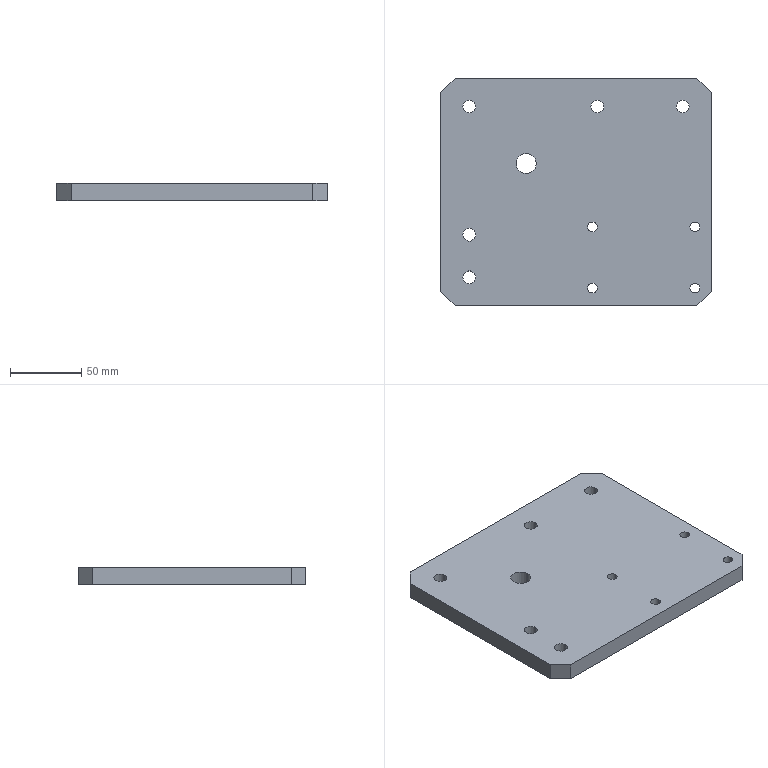Part | SolidWorks | features BaseBody 1 | 1 solid | 30 faces | box 190 x 160 x 12 mm | volume 354993 mm3 | cylinder 20 | plane 10 | commonest cylinder face diameters 9 x10 6.8 x8 14 x2
STEP:
#1=CARTESIAN_POINT('',(181.9,-147.5,15.));
#2=VERTEX_POINT('',#1);
#3=CARTESIAN_POINT('',(175.1,-147.5,15.));
#4=VERTEX_POINT('',#3);
#5=CARTESIAN_POINT('',(178.5,-147.5,15.));
#6=DIRECTION('',(0.,0.,-1.));
#7=DIRECTION('',(-1.,0.,0.));
#8=AXIS2_PLACEMENT_3D('',#5,#6,#7);
#9=CIRCLE('',#8,3.4);
#10=EDGE_CURVE('',#2,#4,#9,.T.);
#11=ORIENTED_EDGE('',*,*,#10,.F.);
#12=CARTESIAN_POINT('',(181.9,-147.5,3.));
#13=VERTEX_POINT('',#12);
#14=CARTESIAN_POINT('',(181.9,-147.5,3.));
#15=DIRECTION('',(0.,0.,-1.));
#16=VECTOR('',#15,1000.);
#17=LINE('',#14,#16);
#18=EDGE_CURVE('',#2,#13,#17,.T.);
#19=ORIENTED_EDGE('',*,*,#18,.T.);
#20=CARTESIAN_POINT('',(175.1,-147.5,3.));
#21=VERTEX_POINT('',#20);
#22=CARTESIAN_POINT('',(178.5,-147.5,3.));
#23=DIRECTION('',(0.,0.,-1.));
#24=DIRECTION('',(-1.,0.,0.));
#25=AXIS2_PLACEMENT_3D('',#22,#23,#24);
#26=CIRCLE('',#25,3.4);
#27=EDGE_CURVE('',#13,#21,#26,.T.);
#28=ORIENTED_EDGE('',*,*,#27,.T.);
#29=CARTESIAN_POINT('',(175.1,-147.5,3.));
#30=DIRECTION('',(0.,0.,-1.));
#31=VECTOR('',#30,1000.);
#32=LINE('',#29,#31);
#33=EDGE_CURVE('',#4,#21,#32,.T.);
#34=ORIENTED_EDGE('',*,*,#33,.F.);
#35=EDGE_LOOP('',(#11,#19,#28,#34));
#36=FACE_OUTER_BOUND('',#35,.T.);
#37=CARTESIAN_POINT('',(178.5,-147.5,3.));
#38=DIRECTION('',(0.,0.,-1.));
#39=DIRECTION('',(-1.,0.,0.));
#40=AXIS2_PLACEMENT_3D('',#37,#38,#39);
#41=CYLINDRICAL_SURFACE('',#40,3.4);
#42=ADVANCED_FACE('',(#36),#41,.F.);
#43=CARTESIAN_POINT('',(181.9,-104.5,15.));
#44=VERTEX_POINT('',#43);
#45=CARTESIAN_POINT('',(175.1,-104.5,15.));
#46=VERTEX_POINT('',#45);
#47=CARTESIAN_POINT('',(178.5,-104.5,15.));
#48=DIRECTION('',(0.,0.,-1.));
#49=DIRECTION('',(-1.,0.,0.));
#50=AXIS2_PLACEMENT_3D('',#47,#48,#49);
#51=CIRCLE('',#50,3.4);
#52=EDGE_CURVE('',#44,#46,#51,.T.);
#53=ORIENTED_EDGE('',*,*,#52,.F.);
#54=CARTESIAN_POINT('',(181.9,-104.5,3.));
#55=VERTEX_POINT('',#54);
#56=CARTESIAN_POINT('',(181.9,-104.5,3.));
#57=DIRECTION('',(0.,0.,-1.));
#58=VECTOR('',#57,1000.);
#59=LINE('',#56,#58);
#60=EDGE_CURVE('',#44,#55,#59,.T.);
#61=ORIENTED_EDGE('',*,*,#60,.T.);
#62=CARTESIAN_POINT('',(175.1,-104.5,3.));
#63=VERTEX_POINT('',#62);
#64=CARTESIAN_POINT('',(178.5,-104.5,3.));
#65=DIRECTION('',(0.,0.,-1.));
#66=DIRECTION('',(-1.,0.,0.));
#67=AXIS2_PLACEMENT_3D('',#64,#65,#66);
#68=CIRCLE('',#67,3.4);
#69=EDGE_CURVE('',#55,#63,#68,.T.);
#70=ORIENTED_EDGE('',*,*,#69,.T.);
#71=CARTESIAN_POINT('',(175.1,-104.5,3.));
#72=DIRECTION('',(0.,0.,-1.));
#73=VECTOR('',#72,1000.);
#74=LINE('',#71,#73);
#75=EDGE_CURVE('',#46,#63,#74,.T.);
#76=ORIENTED_EDGE('',*,*,#75,.F.);
#77=EDGE_LOOP('',(#53,#61,#70,#76));
#78=FACE_OUTER_BOUND('',#77,.T.);
#79=CARTESIAN_POINT('',(178.5,-104.5,3.));
#80=DIRECTION('',(0.,0.,-1.));
#81=DIRECTION('',(-1.,0.,0.));
#82=AXIS2_PLACEMENT_3D('',#79,#80,#81);
#83=CYLINDRICAL_SURFACE('',#82,3.4);
#84=ADVANCED_FACE('',(#78),#83,.F.);
#85=CARTESIAN_POINT('',(109.9,-104.5,15.));
#86=VERTEX_POINT('',#85);
#87=CARTESIAN_POINT('',(103.1,-104.5,15.));
#88=VERTEX_POINT('',#87);
#89=CARTESIAN_POINT('',(106.5,-104.5,15.));
#90=DIRECTION('',(0.,0.,-1.));
#91=DIRECTION('',(-1.,0.,0.));
#92=AXIS2_PLACEMENT_3D('',#89,#90,#91);
#93=CIRCLE('',#92,3.4);
#94=EDGE_CURVE('',#86,#88,#93,.T.);
#95=ORIENTED_EDGE('',*,*,#94,.F.);
#96=CARTESIAN_POINT('',(109.9,-104.5,3.));
#97=VERTEX_POINT('',#96);
#98=CARTESIAN_POINT('',(109.9,-104.5,3.));
#99=DIRECTION('',(0.,0.,-1.));
#100=VECTOR('',#99,1000.);
#101=LINE('',#98,#100);
#102=EDGE_CURVE('',#86,#97,#101,.T.);
#103=ORIENTED_EDGE('',*,*,#102,.T.);
#104=CARTESIAN_POINT('',(103.1,-104.5,3.));
#105=VERTEX_POINT('',#104);
#106=CARTESIAN_POINT('',(106.5,-104.5,3.));
#107=DIRECTION('',(0.,0.,-1.));
#108=DIRECTION('',(-1.,0.,0.));
#109=AXIS2_PLACEMENT_3D('',#106,#107,#108);
#110=CIRCLE('',#109,3.4);
#111=EDGE_CURVE('',#97,#105,#110,.T.);
#112=ORIENTED_EDGE('',*,*,#111,.T.);
#113=CARTESIAN_POINT('',(103.1,-104.5,3.));
#114=DIRECTION('',(0.,0.,-1.));
#115=VECTOR('',#114,1000.);
#116=LINE('',#113,#115);
#117=EDGE_CURVE('',#88,#105,#116,.T.);
#118=ORIENTED_EDGE('',*,*,#117,.F.);
#119=EDGE_LOOP('',(#95,#103,#112,#118));
#120=FACE_OUTER_BOUND('',#119,.T.);
#121=CARTESIAN_POINT('',(106.5,-104.5,3.));
#122=DIRECTION('',(0.,0.,-1.));
#123=DIRECTION('',(-1.,0.,0.));
#124=AXIS2_PLACEMENT_3D('',#121,#122,#123);
#125=CYLINDRICAL_SURFACE('',#124,3.4);
#126=ADVANCED_FACE('',(#120),#125,.F.);
#127=CARTESIAN_POINT('',(109.9,-147.5,15.));
#128=VERTEX_POINT('',#127);
#129=CARTESIAN_POINT('',(103.1,-147.5,15.));
#130=VERTEX_POINT('',#129);
#131=CARTESIAN_POINT('',(106.5,-147.5,15.));
#132=DIRECTION('',(0.,0.,-1.));
#133=DIRECTION('',(-1.,0.,0.));
#134=AXIS2_PLACEMENT_3D('',#131,#132,#133);
#135=CIRCLE('',#134,3.4);
#136=EDGE_CURVE('',#128,#130,#135,.T.);
#137=ORIENTED_EDGE('',*,*,#136,.F.);
#138=CARTESIAN_POINT('',(109.9,-147.5,3.));
#139=VERTEX_POINT('',#138);
#140=CARTESIAN_POINT('',(109.9,-147.5,3.));
#141=DIRECTION('',(0.,0.,-1.));
#142=VECTOR('',#141,1000.);
#143=LINE('',#140,#142);
#144=EDGE_CURVE('',#128,#139,#143,.T.);
#145=ORIENTED_EDGE('',*,*,#144,.T.);
#146=CARTESIAN_POINT('',(103.1,-147.5,3.));
#147=VERTEX_POINT('',#146);
#148=CARTESIAN_POINT('',(106.5,-147.5,3.));
#149=DIRECTION('',(0.,0.,-1.));
#150=DIRECTION('',(-1.,0.,0.));
#151=AXIS2_PLACEMENT_3D('',#148,#149,#150);
#152=CIRCLE('',#151,3.4);
#153=EDGE_CURVE('',#139,#147,#152,.T.);
#154=ORIENTED_EDGE('',*,*,#153,.T.);
#155=CARTESIAN_POINT('',(103.1,-147.5,3.));
#156=DIRECTION('',(0.,0.,-1.));
#157=VECTOR('',#156,1000.);
#158=LINE('',#155,#157);
#159=EDGE_CURVE('',#130,#147,#158,.T.);
#160=ORIENTED_EDGE('',*,*,#159,.F.);
#161=EDGE_LOOP('',(#137,#145,#154,#160));
#162=FACE_OUTER_BOUND('',#161,.T.);
#163=CARTESIAN_POINT('',(106.5,-147.5,3.));
#164=DIRECTION('',(0.,0.,-1.));
#165=DIRECTION('',(-1.,0.,0.));
#166=AXIS2_PLACEMENT_3D('',#163,#164,#165);
#167=CYLINDRICAL_SURFACE('',#166,3.4);
#168=ADVANCED_FACE('',(#162),#167,.F.);
#169=CARTESIAN_POINT('',(67.,-60.,15.));
#170=VERTEX_POINT('',#169);
#171=CARTESIAN_POINT('',(53.,-60.,15.));
#172=VERTEX_POINT('',#171);
#173=CARTESIAN_POINT('',(60.,-60.,15.));
#174=DIRECTION('',(0.,0.,-1.));
#175=DIRECTION('',(-1.,0.,0.));
#176=AXIS2_PLACEMENT_3D('',#173,#174,#175);
#177=CIRCLE('',#176,7.);
#178=EDGE_CURVE('',#170,#172,#177,.T.);
#179=ORIENTED_EDGE('',*,*,#178,.F.);
#180=CARTESIAN_POINT('',(67.,-60.,3.));
#181=VERTEX_POINT('',#180);
#182=CARTESIAN_POINT('',(67.,-60.,3.));
#183=DIRECTION('',(0.,0.,-1.));
#184=VECTOR('',#183,1000.);
#185=LINE('',#182,#184);
#186=EDGE_CURVE('',#170,#181,#185,.T.);
#187=ORIENTED_EDGE('',*,*,#186,.T.);
#188=CARTESIAN_POINT('',(53.,-60.,3.));
#189=VERTEX_POINT('',#188);
#190=CARTESIAN_POINT('',(60.,-60.,3.));
#191=DIRECTION('',(0.,0.,-1.));
#192=DIRECTION('',(-1.,0.,0.));
#193=AXIS2_PLACEMENT_3D('',#190,#191,#192);
#194=CIRCLE('',#193,7.);
#195=EDGE_CURVE('',#181,#189,#194,.T.);
#196=ORIENTED_EDGE('',*,*,#195,.T.);
#197=CARTESIAN_POINT('',(53.,-60.,3.));
#198=DIRECTION('',(0.,0.,-1.));
#199=VECTOR('',#198,1000.);
#200=LINE('',#197,#199);
#201=EDGE_CURVE('',#172,#189,#200,.T.);
#202=ORIENTED_EDGE('',*,*,#201,.F.);
#203=EDGE_LOOP('',(#179,#187,#196,#202));
#204=FACE_OUTER_BOUND('',#203,.T.);
#205=CARTESIAN_POINT('',(60.,-60.,3.));
#206=DIRECTION('',(0.,0.,-1.));
#207=DIRECTION('',(-1.,0.,0.));
#208=AXIS2_PLACEMENT_3D('',#205,#206,#207);
#209=CYLINDRICAL_SURFACE('',#208,7.);
#210=ADVANCED_FACE('',(#204),#209,.F.);
#211=CARTESIAN_POINT('',(15.5,-20.,3.));
#212=VERTEX_POINT('',#211);
#213=CARTESIAN_POINT('',(24.5,-20.,3.));
#214=VERTEX_POINT('',#213);
#215=CARTESIAN_POINT('',(20.,-20.,3.));
#216=DIRECTION('',(0.,0.,1.));
#217=DIRECTION('',(1.,0.,0.));
#218=AXIS2_PLACEMENT_3D('',#215,#216,#217);
#219=CIRCLE('',#218,4.5);
#220=EDGE_CURVE('',#212,#214,#219,.T.);
#221=ORIENTED_EDGE('',*,*,#220,.F.);
#222=CARTESIAN_POINT('',(15.5,-20.,15.));
#223=VERTEX_POINT('',#222);
#224=CARTESIAN_POINT('',(15.5,-20.,15.));
#225=DIRECTION('',(0.,0.,1.));
#226=VECTOR('',#225,1000.);
#227=LINE('',#224,#226);
#228=EDGE_CURVE('',#212,#223,#227,.T.);
#229=ORIENTED_EDGE('',*,*,#228,.T.);
#230=CARTESIAN_POINT('',(24.5,-20.,15.));
#231=VERTEX_POINT('',#230);
#232=CARTESIAN_POINT('',(20.,-20.,15.));
#233=DIRECTION('',(0.,0.,1.));
#234=DIRECTION('',(1.,0.,0.));
#235=AXIS2_PLACEMENT_3D('',#232,#233,#234);
#236=CIRCLE('',#235,4.5);
#237=EDGE_CURVE('',#223,#231,#236,.T.);
#238=ORIENTED_EDGE('',*,*,#237,.T.);
#239=CARTESIAN_POINT('',(24.5,-20.,15.));
#240=DIRECTION('',(0.,0.,1.));
#241=VECTOR('',#240,1000.);
#242=LINE('',#239,#241);
#243=EDGE_CURVE('',#214,#231,#242,.T.);
#244=ORIENTED_EDGE('',*,*,#243,.F.);
#245=EDGE_LOOP('',(#221,#229,#238,#244));
#246=FACE_OUTER_BOUND('',#245,.T.);
#247=CARTESIAN_POINT('',(20.,-20.,15.));
#248=DIRECTION('',(0.,0.,1.));
#249=DIRECTION('',(1.,0.,0.));
#250=AXIS2_PLACEMENT_3D('',#247,#248,#249);
#251=CYLINDRICAL_SURFACE('',#250,4.5);
#252=ADVANCED_FACE('',(#246),#251,.F.);
#253=CARTESIAN_POINT('',(105.5,-20.,3.));
#254=VERTEX_POINT('',#253);
#255=CARTESIAN_POINT('',(114.5,-20.,3.));
#256=VERTEX_POINT('',#255);
#257=CARTESIAN_POINT('',(110.,-20.,3.));
#258=DIRECTION('',(0.,0.,1.));
#259=DIRECTION('',(1.,0.,0.));
#260=AXIS2_PLACEMENT_3D('',#257,#258,#259);
#261=CIRCLE('',#260,4.5);
#262=EDGE_CURVE('',#254,#256,#261,.T.);
#263=ORIENTED_EDGE('',*,*,#262,.F.);
#264=CARTESIAN_POINT('',(105.5,-20.,15.));
#265=VERTEX_POINT('',#264);
#266=CARTESIAN_POINT('',(105.5,-20.,15.));
#267=DIRECTION('',(0.,0.,1.));
#268=VECTOR('',#267,1000.);
#269=LINE('',#266,#268);
#270=EDGE_CURVE('',#254,#265,#269,.T.);
#271=ORIENTED_EDGE('',*,*,#270,.T.);
#272=CARTESIAN_POINT('',(114.5,-20.,15.));
#273=VERTEX_POINT('',#272);
#274=CARTESIAN_POINT('',(110.,-20.,15.));
#275=DIRECTION('',(0.,0.,1.));
#276=DIRECTION('',(1.,0.,0.));
#277=AXIS2_PLACEMENT_3D('',#274,#275,#276);
#278=CIRCLE('',#277,4.5);
#279=EDGE_CURVE('',#265,#273,#278,.T.);
#280=ORIENTED_EDGE('',*,*,#279,.T.);
#281=CARTESIAN_POINT('',(114.5,-20.,15.));
#282=DIRECTION('',(0.,0.,1.));
#283=VECTOR('',#282,1000.);
#284=LINE('',#281,#283);
#285=EDGE_CURVE('',#256,#273,#284,.T.);
#286=ORIENTED_EDGE('',*,*,#285,.F.);
#287=EDGE_LOOP('',(#263,#271,#280,#286));
#288=FACE_OUTER_BOUND('',#287,.T.);
#289=CARTESIAN_POINT('',(110.,-20.,15.));
#290=DIRECTION('',(0.,0.,1.));
#291=DIRECTION('',(1.,0.,0.));
#292=AXIS2_PLACEMENT_3D('',#289,#290,#291);
#293=CYLINDRICAL_SURFACE('',#292,4.5);
#294=ADVANCED_FACE('',(#288),#293,.F.);
#295=CARTESIAN_POINT('',(165.5,-20.,3.));
#296=VERTEX_POINT('',#295);
#297=CARTESIAN_POINT('',(174.5,-20.,3.));
#298=VERTEX_POINT('',#297);
#299=CARTESIAN_POINT('',(170.,-20.,3.));
#300=DIRECTION('',(0.,0.,1.));
#301=DIRECTION('',(1.,0.,0.));
#302=AXIS2_PLACEMENT_3D('',#299,#300,#301);
#303=CIRCLE('',#302,4.5);
#304=EDGE_CURVE('',#296,#298,#303,.T.);
#305=ORIENTED_EDGE('',*,*,#304,.F.);
#306=CARTESIAN_POINT('',(165.5,-20.,15.));
#307=VERTEX_POINT('',#306);
#308=CARTESIAN_POINT('',(165.5,-20.,15.));
#309=DIRECTION('',(0.,0.,1.));
#310=VECTOR('',#309,1000.);
#311=LINE('',#308,#310);
#312=EDGE_CURVE('',#296,#307,#311,.T.);
#313=ORIENTED_EDGE('',*,*,#312,.T.);
#314=CARTESIAN_POINT('',(174.5,-20.,15.));
#315=VERTEX_POINT('',#314);
#316=CARTESIAN_POINT('',(170.,-20.,15.));
#317=DIRECTION('',(0.,0.,1.));
#318=DIRECTION('',(1.,0.,0.));
#319=AXIS2_PLACEMENT_3D('',#316,#317,#318);
#320=CIRCLE('',#319,4.5);
#321=EDGE_CURVE('',#307,#315,#320,.T.);
#322=ORIENTED_EDGE('',*,*,#321,.T.);
#323=CARTESIAN_POINT('',(174.5,-20.,15.));
#324=DIRECTION('',(0.,0.,1.));
#325=VECTOR('',#324,1000.);
#326=LINE('',#323,#325);
#327=EDGE_CURVE('',#298,#315,#326,.T.);
#328=ORIENTED_EDGE('',*,*,#327,.F.);
#329=EDGE_LOOP('',(#305,#313,#322,#328));
#330=FACE_OUTER_BOUND('',#329,.T.);
#331=CARTESIAN_POINT('',(170.,-20.,15.));
#332=DIRECTION('',(0.,0.,1.));
#333=DIRECTION('',(1.,0.,0.));
#334=AXIS2_PLACEMENT_3D('',#331,#332,#333);
#335=CYLINDRICAL_SURFACE('',#334,4.5);
#336=ADVANCED_FACE('',(#330),#335,.F.);
#337=CARTESIAN_POINT('',(15.5,-110.,3.));
#338=VERTEX_POINT('',#337);
#339=CARTESIAN_POINT('',(24.5,-110.,3.));
#340=VERTEX_POINT('',#339);
#341=CARTESIAN_POINT('',(20.,-110.,3.));
#342=DIRECTION('',(0.,0.,1.));
#343=DIRECTION('',(1.,0.,0.));
#344=AXIS2_PLACEMENT_3D('',#341,#342,#343);
#345=CIRCLE('',#344,4.5);
#346=EDGE_CURVE('',#338,#340,#345,.T.);
#347=ORIENTED_EDGE('',*,*,#346,.F.);
#348=CARTESIAN_POINT('',(15.5,-110.,15.));
#349=VERTEX_POINT('',#348);
#350=CARTESIAN_POINT('',(15.5,-110.,15.));
#351=DIRECTION('',(0.,0.,1.));
#352=VECTOR('',#351,1000.);
#353=LINE('',#350,#352);
#354=EDGE_CURVE('',#338,#349,#353,.T.);
#355=ORIENTED_EDGE('',*,*,#354,.T.);
#356=CARTESIAN_POINT('',(24.5,-110.,15.));
#357=VERTEX_POINT('',#356);
#358=CARTESIAN_POINT('',(20.,-110.,15.));
#359=DIRECTION('',(0.,0.,1.));
#360=DIRECTION('',(1.,0.,0.));
#361=AXIS2_PLACEMENT_3D('',#358,#359,#360);
#362=CIRCLE('',#361,4.5);
#363=EDGE_CURVE('',#349,#357,#362,.T.);
#364=ORIENTED_EDGE('',*,*,#363,.T.);
#365=CARTESIAN_POINT('',(24.5,-110.,15.));
#366=DIRECTION('',(0.,0.,1.));
#367=VECTOR('',#366,1000.);
#368=LINE('',#365,#367);
#369=EDGE_CURVE('',#340,#357,#368,.T.);
#370=ORIENTED_EDGE('',*,*,#369,.F.);
#371=EDGE_LOOP('',(#347,#355,#364,#370));
#372=FACE_OUTER_BOUND('',#371,.T.);
#373=CARTESIAN_POINT('',(20.,-110.,15.));
#374=DIRECTION('',(0.,0.,1.));
#375=DIRECTION('',(1.,0.,0.));
#376=AXIS2_PLACEMENT_3D('',#373,#374,#375);
#377=CYLINDRICAL_SURFACE('',#376,4.5);
#378=ADVANCED_FACE('',(#372),#377,.F.);
#379=CARTESIAN_POINT('',(15.5,-140.,3.));
#380=VERTEX_POINT('',#379);
#381=CARTESIAN_POINT('',(24.5,-140.,3.));
#382=VERTEX_POINT('',#381);
#383=CARTESIAN_POINT('',(20.,-140.,3.));
#384=DIRECTION('',(0.,0.,1.));
#385=DIRECTION('',(1.,0.,0.));
#386=AXIS2_PLACEMENT_3D('',#383,#384,#385);
#387=CIRCLE('',#386,4.5);
#388=EDGE_CURVE('',#380,#382,#387,.T.);
#389=ORIENTED_EDGE('',*,*,#388,.F.);
#390=CARTESIAN_POINT('',(15.5,-140.,15.));
#391=VERTEX_POINT('',#390);
#392=CARTESIAN_POINT('',(15.5,-140.,15.));
#393=DIRECTION('',(0.,0.,1.));
#394=VECTOR('',#393,1000.);
#395=LINE('',#392,#394);
#396=EDGE_CURVE('',#380,#391,#395,.T.);
#397=ORIENTED_EDGE('',*,*,#396,.T.);
#398=CARTESIAN_POINT('',(24.5,-140.,15.));
#399=VERTEX_POINT('',#398);
#400=CARTESIAN_POINT('',(20.,-140.,15.));
#401=DIRECTION('',(0.,0.,1.));
#402=DIRECTION('',(1.,0.,0.));
#403=AXIS2_PLACEMENT_3D('',#400,#401,#402);
#404=CIRCLE('',#403,4.5);
#405=EDGE_CURVE('',#391,#399,#404,.T.);
#406=ORIENTED_EDGE('',*,*,#405,.T.);
#407=CARTESIAN_POINT('',(24.5,-140.,15.));
#408=DIRECTION('',(0.,0.,1.));
#409=VECTOR('',#408,1000.);
#410=LINE('',#407,#409);
#411=EDGE_CURVE('',#382,#399,#410,.T.);
#412=ORIENTED_EDGE('',*,*,#411,.F.);
#413=EDGE_LOOP('',(#389,#397,#406,#412));
#414=FACE_OUTER_BOUND('',#413,.T.);
#415=CARTESIAN_POINT('',(20.,-140.,15.));
#416=DIRECTION('',(0.,0.,1.));
#417=DIRECTION('',(1.,0.,0.));
#418=AXIS2_PLACEMENT_3D('',#415,#416,#417);
#419=CYLINDRICAL_SURFACE('',#418,4.5);
#420=ADVANCED_FACE('',(#414),#419,.F.);
#421=CARTESIAN_POINT('',(180.,0.,3.));
#422=VERTEX_POINT('',#421);
#423=CARTESIAN_POINT('',(10.,0.,3.));
#424=VERTEX_POINT('',#423);
#425=CARTESIAN_POINT('',(190.,0.,3.));
#426=DIRECTION('',(-1.,0.,0.));
#427=VECTOR('',#426,1000.);
#428=LINE('',#425,#427);
#429=EDGE_CURVE('',#422,#424,#428,.T.);
#430=ORIENTED_EDGE('',*,*,#429,.T.);
#431=CARTESIAN_POINT('',(10.,0.,15.));
#432=VERTEX_POINT('',#431);
#433=CARTESIAN_POINT('',(10.,0.,3.));
#434=DIRECTION('',(0.,0.,1.));
#435=VECTOR('',#434,1000.);
#436=LINE('',#433,#435);
#437=EDGE_CURVE('',#424,#432,#436,.T.);
#438=ORIENTED_EDGE('',*,*,#437,.T.);
#439=CARTESIAN_POINT('',(180.,0.,15.));
#440=VERTEX_POINT('',#439);
#441=CARTESIAN_POINT('',(190.,0.,15.));
#442=DIRECTION('',(-1.,0.,0.));
#443=VECTOR('',#442,1000.);
#444=LINE('',#441,#443);
#445=EDGE_CURVE('',#440,#432,#444,.T.);
#446=ORIENTED_EDGE('',*,*,#445,.F.);
#447=CARTESIAN_POINT('',(180.,0.,3.));
#448=DIRECTION('',(0.,0.,-1.));
#449=VECTOR('',#448,1000.);
#450=LINE('',#447,#449);
#451=EDGE_CURVE('',#440,#422,#450,.T.);
#452=ORIENTED_EDGE('',*,*,#451,.T.);
#453=EDGE_LOOP('',(#430,#438,#446,#452));
#454=FACE_OUTER_BOUND('',#453,.T.);
#455=CARTESIAN_POINT('',(190.,0.,3.));
#456=DIRECTION('',(0.,1.,0.));
#457=DIRECTION('',(-1.,0.,0.));
#458=AXIS2_PLACEMENT_3D('',#455,#456,#457);
#459=PLANE('',#458);
#460=ADVANCED_FACE('',(#454),#459,.T.);
#461=CARTESIAN_POINT('',(190.,-150.,3.));
#462=VERTEX_POINT('',#461);
#463=CARTESIAN_POINT('',(190.,-10.,3.));
#464=VERTEX_POINT('',#463);
#465=CARTESIAN_POINT('',(190.,-160.,3.));
#466=DIRECTION('',(0.,1.,0.));
#467=VECTOR('',#466,1000.);
#468=LINE('',#465,#467);
#469=EDGE_CURVE('',#462,#464,#468,.T.);
#470=ORIENTED_EDGE('',*,*,#469,.T.);
#471=CARTESIAN_POINT('',(190.,-10.,15.));
#472=VERTEX_POINT('',#471);
#473=CARTESIAN_POINT('',(190.,-10.,3.));
#474=DIRECTION('',(0.,0.,1.));
#475=VECTOR('',#474,1000.);
#476=LINE('',#473,#475);
#477=EDGE_CURVE('',#464,#472,#476,.T.);
#478=ORIENTED_EDGE('',*,*,#477,.T.);
#479=CARTESIAN_POINT('',(190.,-150.,15.));
#480=VERTEX_POINT('',#479);
#481=CARTESIAN_POINT('',(190.,-160.,15.));
#482=DIRECTION('',(0.,1.,0.));
#483=VECTOR('',#482,1000.);
#484=LINE('',#481,#483);
#485=EDGE_CURVE('',#480,#472,#484,.T.);
#486=ORIENTED_EDGE('',*,*,#485,.F.);
#487=CARTESIAN_POINT('',(190.,-150.,3.));
#488=DIRECTION('',(0.,0.,-1.));
#489=VECTOR('',#488,1000.);
#490=LINE('',#487,#489);
#491=EDGE_CURVE('',#480,#462,#490,.T.);
#492=ORIENTED_EDGE('',*,*,#491,.T.);
#493=EDGE_LOOP('',(#470,#478,#486,#492));
#494=FACE_OUTER_BOUND('',#493,.T.);
#495=CARTESIAN_POINT('',(190.,-160.,3.));
#496=DIRECTION('',(1.,0.,0.));
#497=DIRECTION('',(0.,0.,-1.));
#498=AXIS2_PLACEMENT_3D('',#495,#496,#497);
#499=PLANE('',#498);
#500=ADVANCED_FACE('',(#494),#499,.T.);
#501=CARTESIAN_POINT('',(10.,-160.,3.));
#502=VERTEX_POINT('',#501);
#503=CARTESIAN_POINT('',(180.,-160.,3.));
#504=VERTEX_POINT('',#503);
#505=CARTESIAN_POINT('',(0.,-160.,3.));
#506=DIRECTION('',(1.,0.,0.));
#507=VECTOR('',#506,1000.);
#508=LINE('',#505,#507);
#509=EDGE_CURVE('',#502,#504,#508,.T.);
#510=ORIENTED_EDGE('',*,*,#509,.T.);
#511=CARTESIAN_POINT('',(180.,-160.,15.));
#512=VERTEX_POINT('',#511);
#513=CARTESIAN_POINT('',(180.,-160.,3.));
#514=DIRECTION('',(0.,0.,1.));
#515=VECTOR('',#514,1000.);
#516=LINE('',#513,#515);
#517=EDGE_CURVE('',#504,#512,#516,.T.);
#518=ORIENTED_EDGE('',*,*,#517,.T.);
#519=CARTESIAN_POINT('',(10.,-160.,15.));
#520=VERTEX_POINT('',#519);
#521=CARTESIAN_POINT('',(0.,-160.,15.));
#522=DIRECTION('',(1.,0.,0.));
#523=VECTOR('',#522,1000.);
#524=LINE('',#521,#523);
#525=EDGE_CURVE('',#520,#512,#524,.T.);
#526=ORIENTED_EDGE('',*,*,#525,.F.);
#527=CARTESIAN_POINT('',(10.,-160.,3.));
#528=DIRECTION('',(0.,0.,-1.));
#529=VECTOR('',#528,1000.);
#530=LINE('',#527,#529);
#531=EDGE_CURVE('',#520,#502,#530,.T.);
#532=ORIENTED_EDGE('',*,*,#531,.T.);
#533=EDGE_LOOP('',(#510,#518,#526,#532));
#534=FACE_OUTER_BOUND('',#533,.T.);
#535=CARTESIAN_POINT('',(0.,-160.,3.));
#536=DIRECTION('',(0.,-1.,0.));
#537=DIRECTION('',(0.,0.,-1.));
#538=AXIS2_PLACEMENT_3D('',#535,#536,#537);
#539=PLANE('',#538);
#540=ADVANCED_FACE('',(#534),#539,.T.);
#541=CARTESIAN_POINT('',(0.,-10.,15.));
#542=VERTEX_POINT('',#541);
#543=CARTESIAN_POINT('',(0.,-150.,15.));
#544=VERTEX_POINT('',#543);
#545=CARTESIAN_POINT('',(0.,0.,15.));
#546=DIRECTION('',(0.,-1.,0.));
#547=VECTOR('',#546,1000.);
#548=LINE('',#545,#547);
#549=EDGE_CURVE('',#542,#544,#548,.T.);
#550=ORIENTED_EDGE('',*,*,#549,.F.);
#551=CARTESIAN_POINT('',(0.,-10.,3.));
#552=VERTEX_POINT('',#551);
#553=CARTESIAN_POINT('',(0.,-10.,3.));
#554=DIRECTION('',(0.,0.,-1.));
#555=VECTOR('',#554,1000.);
#556=LINE('',#553,#555);
#557=EDGE_CURVE('',#542,#552,#556,.T.);
#558=ORIENTED_EDGE('',*,*,#557,.T.);
#559=CARTESIAN_POINT('',(0.,-150.,3.));
#560=VERTEX_POINT('',#559);
#561=CARTESIAN_POINT('',(0.,0.,3.));
#562=DIRECTION('',(0.,-1.,0.));
#563=VECTOR('',#562,1000.);
#564=LINE('',#561,#563);
#565=EDGE_CURVE('',#552,#560,#564,.T.);
#566=ORIENTED_EDGE('',*,*,#565,.T.);
#567=CARTESIAN_POINT('',(0.,-150.,3.));
#568=DIRECTION('',(0.,0.,1.));
#569=VECTOR('',#568,1000.);
#570=LINE('',#567,#569);
#571=EDGE_CURVE('',#560,#544,#570,.T.);
#572=ORIENTED_EDGE('',*,*,#571,.T.);
#573=EDGE_LOOP('',(#550,#558,#566,#572));
#574=FACE_OUTER_BOUND('',#573,.T.);
#575=CARTESIAN_POINT('',(0.,0.,3.));
#576=DIRECTION('',(-1.,0.,0.));
#577=DIRECTION('',(0.,-1.,0.));
#578=AXIS2_PLACEMENT_3D('',#575,#576,#577);
#579=PLANE('',#578);
#580=ADVANCED_FACE('',(#574),#579,.T.);
#581=CARTESIAN_POINT('',(178.5,-147.5,3.));
#582=DIRECTION('',(0.,0.,-1.));
#583=DIRECTION('',(-1.,0.,0.));
#584=AXIS2_PLACEMENT_3D('',#581,#582,#583);
#585=CIRCLE('',#584,3.4);
#586=EDGE_CURVE('',#21,#13,#585,.T.);
#587=ORIENTED_EDGE('',*,*,#586,.F.);
#588=ORIENTED_EDGE('',*,*,#27,.F.);
#589=EDGE_LOOP('',(#587,#588));
#590=FACE_BOUND('',#589,.T.);
#591=CARTESIAN_POINT('',(178.5,-104.5,3.));
#592=DIRECTION('',(0.,0.,-1.));
#593=DIRECTION('',(-1.,0.,0.));
#594=AXIS2_PLACEMENT_3D('',#591,#592,#593);
#595=CIRCLE('',#594,3.4);
#596=EDGE_CURVE('',#63,#55,#595,.T.);
#597=ORIENTED_EDGE('',*,*,#596,.F.);
#598=ORIENTED_EDGE('',*,*,#69,.F.);
#599=EDGE_LOOP('',(#597,#598));
#600=FACE_BOUND('',#599,.T.);
#601=CARTESIAN_POINT('',(106.5,-104.5,3.));
#602=DIRECTION('',(0.,0.,-1.));
#603=DIRECTION('',(-1.,0.,0.));
#604=AXIS2_PLACEMENT_3D('',#601,#602,#603);
#605=CIRCLE('',#604,3.4);
#606=EDGE_CURVE('',#105,#97,#605,.T.);
#607=ORIENTED_EDGE('',*,*,#606,.F.);
#608=ORIENTED_EDGE('',*,*,#111,.F.);
#609=EDGE_LOOP('',(#607,#608));
#610=FACE_BOUND('',#609,.T.);
#611=CARTESIAN_POINT('',(106.5,-147.5,3.));
#612=DIRECTION('',(0.,0.,-1.));
#613=DIRECTION('',(-1.,0.,0.));
#614=AXIS2_PLACEMENT_3D('',#611,#612,#613);
#615=CIRCLE('',#614,3.4);
#616=EDGE_CURVE('',#147,#139,#615,.T.);
#617=ORIENTED_EDGE('',*,*,#616,.F.);
#618=ORIENTED_EDGE('',*,*,#153,.F.);
#619=EDGE_LOOP('',(#617,#618));
#620=FACE_BOUND('',#619,.T.);
#621=CARTESIAN_POINT('',(60.,-60.,3.));
#622=DIRECTION('',(0.,0.,-1.));
#623=DIRECTION('',(-1.,0.,0.));
#624=AXIS2_PLACEMENT_3D('',#621,#622,#623);
#625=CIRCLE('',#624,7.);
#626=EDGE_CURVE('',#189,#181,#625,.T.);
#627=ORIENTED_EDGE('',*,*,#626,.F.);
#628=ORIENTED_EDGE('',*,*,#195,.F.);
#629=EDGE_LOOP('',(#627,#628));
#630=FACE_BOUND('',#629,.T.);
#631=CARTESIAN_POINT('',(20.,-20.,3.));
#632=DIRECTION('',(0.,0.,1.));
#633=DIRECTION('',(1.,0.,0.));
#634=AXIS2_PLACEMENT_3D('',#631,#632,#633);
#635=CIRCLE('',#634,4.5);
#636=EDGE_CURVE('',#214,#212,#635,.T.);
#637=ORIENTED_EDGE('',*,*,#636,.T.);
#638=ORIENTED_EDGE('',*,*,#220,.T.);
#639=EDGE_LOOP('',(#637,#638));
#640=FACE_BOUND('',#639,.T.);
#641=CARTESIAN_POINT('',(110.,-20.,3.));
#642=DIRECTION('',(0.,0.,1.));
#643=DIRECTION('',(1.,0.,0.));
#644=AXIS2_PLACEMENT_3D('',#641,#642,#643);
#645=CIRCLE('',#644,4.5);
#646=EDGE_CURVE('',#256,#254,#645,.T.);
#647=ORIENTED_EDGE('',*,*,#646,.T.);
#648=ORIENTED_EDGE('',*,*,#262,.T.);
#649=EDGE_LOOP('',(#647,#648));
#650=FACE_BOUND('',#649,.T.);
#651=CARTESIAN_POINT('',(170.,-20.,3.));
#652=DIRECTION('',(0.,0.,1.));
#653=DIRECTION('',(1.,0.,0.));
#654=AXIS2_PLACEMENT_3D('',#651,#652,#653);
#655=CIRCLE('',#654,4.5);
#656=EDGE_CURVE('',#298,#296,#655,.T.);
#657=ORIENTED_EDGE('',*,*,#656,.T.);
#658=ORIENTED_EDGE('',*,*,#304,.T.);
#659=EDGE_LOOP('',(#657,#658));
#660=FACE_BOUND('',#659,.T.);
#661=CARTESIAN_POINT('',(20.,-110.,3.));
#662=DIRECTION('',(0.,0.,1.));
#663=DIRECTION('',(1.,0.,0.));
#664=AXIS2_PLACEMENT_3D('',#661,#662,#663);
#665=CIRCLE('',#664,4.5);
#666=EDGE_CURVE('',#340,#338,#665,.T.);
#667=ORIENTED_EDGE('',*,*,#666,.T.);
#668=ORIENTED_EDGE('',*,*,#346,.T.);
#669=EDGE_LOOP('',(#667,#668));
#670=FACE_BOUND('',#669,.T.);
#671=CARTESIAN_POINT('',(20.,-140.,3.));
#672=DIRECTION('',(0.,0.,1.));
#673=DIRECTION('',(1.,0.,0.));
#674=AXIS2_PLACEMENT_3D('',#671,#672,#673);
#675=CIRCLE('',#674,4.5);
#676=EDGE_CURVE('',#382,#380,#675,.T.);
#677=ORIENTED_EDGE('',*,*,#676,.T.);
#678=ORIENTED_EDGE('',*,*,#388,.T.);
#679=EDGE_LOOP('',(#677,#678));
#680=FACE_BOUND('',#679,.T.);
#681=ORIENTED_EDGE('',*,*,#565,.F.);
#682=CARTESIAN_POINT('',(10.,0.,3.));
#683=DIRECTION('',(0.7071,0.7071,0.));
#684=VECTOR('',#683,1000.);
#685=LINE('',#682,#684);
#686=EDGE_CURVE('',#552,#424,#685,.T.);
#687=ORIENTED_EDGE('',*,*,#686,.T.);
#688=ORIENTED_EDGE('',*,*,#429,.F.);
#689=CARTESIAN_POINT('',(190.,-10.,3.));
#690=DIRECTION('',(0.7071,-0.7071,0.));
#691=VECTOR('',#690,1000.);
#692=LINE('',#689,#691);
#693=EDGE_CURVE('',#422,#464,#692,.T.);
#694=ORIENTED_EDGE('',*,*,#693,.T.);
#695=ORIENTED_EDGE('',*,*,#469,.F.);
#696=CARTESIAN_POINT('',(180.,-160.,3.));
#697=DIRECTION('',(-0.7071,-0.7071,0.));
#698=VECTOR('',#697,1000.);
#699=LINE('',#696,#698);
#700=EDGE_CURVE('',#462,#504,#699,.T.);
#701=ORIENTED_EDGE('',*,*,#700,.T.);
#702=ORIENTED_EDGE('',*,*,#509,.F.);
#703=CARTESIAN_POINT('',(0.,-150.,3.));
#704=DIRECTION('',(-0.7071,0.7071,0.));
#705=VECTOR('',#704,1000.);
#706=LINE('',#703,#705);
#707=EDGE_CURVE('',#502,#560,#706,.T.);
#708=ORIENTED_EDGE('',*,*,#707,.T.);
#709=EDGE_LOOP('',(#681,#687,#688,#694,#695,#701,#702,#708));
#710=FACE_OUTER_BOUND('',#709,.T.);
#711=CARTESIAN_POINT('',(0.,0.,3.));
#712=DIRECTION('',(0.,0.,1.));
#713=DIRECTION('',(1.,0.,0.));
#714=AXIS2_PLACEMENT_3D('',#711,#712,#713);
#715=PLANE('',#714);
#716=ADVANCED_FACE('',(#590,#600,#610,#620,#630,#640,#650,#660,#670,#680,#710),#715,.F.);
#717=CARTESIAN_POINT('',(178.5,-147.5,15.));
#718=DIRECTION('',(0.,0.,-1.));
#719=DIRECTION('',(-1.,0.,0.));
#720=AXIS2_PLACEMENT_3D('',#717,#718,#719);
#721=CIRCLE('',#720,3.4);
#722=EDGE_CURVE('',#4,#2,#721,.T.);
#723=ORIENTED_EDGE('',*,*,#722,.T.);
#724=ORIENTED_EDGE('',*,*,#10,.T.);
#725=EDGE_LOOP('',(#723,#724));
#726=FACE_BOUND('',#725,.T.);
#727=CARTESIAN_POINT('',(178.5,-104.5,15.));
#728=DIRECTION('',(0.,0.,-1.));
#729=DIRECTION('',(-1.,0.,0.));
#730=AXIS2_PLACEMENT_3D('',#727,#728,#729);
#731=CIRCLE('',#730,3.4);
#732=EDGE_CURVE('',#46,#44,#731,.T.);
#733=ORIENTED_EDGE('',*,*,#732,.T.);
#734=ORIENTED_EDGE('',*,*,#52,.T.);
#735=EDGE_LOOP('',(#733,#734));
#736=FACE_BOUND('',#735,.T.);
#737=CARTESIAN_POINT('',(106.5,-104.5,15.));
#738=DIRECTION('',(0.,0.,-1.));
#739=DIRECTION('',(-1.,0.,0.));
#740=AXIS2_PLACEMENT_3D('',#737,#738,#739);
#741=CIRCLE('',#740,3.4);
#742=EDGE_CURVE('',#88,#86,#741,.T.);
#743=ORIENTED_EDGE('',*,*,#742,.T.);
#744=ORIENTED_EDGE('',*,*,#94,.T.);
#745=EDGE_LOOP('',(#743,#744));
#746=FACE_BOUND('',#745,.T.);
#747=CARTESIAN_POINT('',(106.5,-147.5,15.));
#748=DIRECTION('',(0.,0.,-1.));
#749=DIRECTION('',(-1.,0.,0.));
#750=AXIS2_PLACEMENT_3D('',#747,#748,#749);
#751=CIRCLE('',#750,3.4);
#752=EDGE_CURVE('',#130,#128,#751,.T.);
#753=ORIENTED_EDGE('',*,*,#752,.T.);
#754=ORIENTED_EDGE('',*,*,#136,.T.);
#755=EDGE_LOOP('',(#753,#754));
#756=FACE_BOUND('',#755,.T.);
#757=CARTESIAN_POINT('',(60.,-60.,15.));
#758=DIRECTION('',(0.,0.,-1.));
#759=DIRECTION('',(-1.,0.,0.));
#760=AXIS2_PLACEMENT_3D('',#757,#758,#759);
#761=CIRCLE('',#760,7.);
#762=EDGE_CURVE('',#172,#170,#761,.T.);
#763=ORIENTED_EDGE('',*,*,#762,.T.);
#764=ORIENTED_EDGE('',*,*,#178,.T.);
#765=EDGE_LOOP('',(#763,#764));
#766=FACE_BOUND('',#765,.T.);
#767=CARTESIAN_POINT('',(20.,-20.,15.));
#768=DIRECTION('',(0.,0.,1.));
#769=DIRECTION('',(1.,0.,0.));
#770=AXIS2_PLACEMENT_3D('',#767,#768,#769);
#771=CIRCLE('',#770,4.5);
#772=EDGE_CURVE('',#231,#223,#771,.T.);
#773=ORIENTED_EDGE('',*,*,#772,.F.);
#774=ORIENTED_EDGE('',*,*,#237,.F.);
#775=EDGE_LOOP('',(#773,#774));
#776=FACE_BOUND('',#775,.T.);
#777=CARTESIAN_POINT('',(110.,-20.,15.));
#778=DIRECTION('',(0.,0.,1.));
#779=DIRECTION('',(1.,0.,0.));
#780=AXIS2_PLACEMENT_3D('',#777,#778,#779);
#781=CIRCLE('',#780,4.5);
#782=EDGE_CURVE('',#273,#265,#781,.T.);
#783=ORIENTED_EDGE('',*,*,#782,.F.);
#784=ORIENTED_EDGE('',*,*,#279,.F.);
#785=EDGE_LOOP('',(#783,#784));
#786=FACE_BOUND('',#785,.T.);
#787=CARTESIAN_POINT('',(170.,-20.,15.));
#788=DIRECTION('',(0.,0.,1.));
#789=DIRECTION('',(1.,0.,0.));
#790=AXIS2_PLACEMENT_3D('',#787,#788,#789);
#791=CIRCLE('',#790,4.5);
#792=EDGE_CURVE('',#315,#307,#791,.T.);
#793=ORIENTED_EDGE('',*,*,#792,.F.);
#794=ORIENTED_EDGE('',*,*,#321,.F.);
#795=EDGE_LOOP('',(#793,#794));
#796=FACE_BOUND('',#795,.T.);
#797=CARTESIAN_POINT('',(20.,-110.,15.));
#798=DIRECTION('',(0.,0.,1.));
#799=DIRECTION('',(1.,0.,0.));
#800=AXIS2_PLACEMENT_3D('',#797,#798,#799);
#801=CIRCLE('',#800,4.5);
#802=EDGE_CURVE('',#357,#349,#801,.T.);
#803=ORIENTED_EDGE('',*,*,#802,.F.);
#804=ORIENTED_EDGE('',*,*,#363,.F.);
#805=EDGE_LOOP('',(#803,#804));
#806=FACE_BOUND('',#805,.T.);
#807=CARTESIAN_POINT('',(20.,-140.,15.));
#808=DIRECTION('',(0.,0.,1.));
#809=DIRECTION('',(1.,0.,0.));
#810=AXIS2_PLACEMENT_3D('',#807,#808,#809);
#811=CIRCLE('',#810,4.5);
#812=EDGE_CURVE('',#399,#391,#811,.T.);
#813=ORIENTED_EDGE('',*,*,#812,.F.);
#814=ORIENTED_EDGE('',*,*,#405,.F.);
#815=EDGE_LOOP('',(#813,#814));
#816=FACE_BOUND('',#815,.T.);
#817=ORIENTED_EDGE('',*,*,#445,.T.);
#818=CARTESIAN_POINT('',(5.,-5.,15.));
#819=DIRECTION('',(-0.7071,-0.7071,0.));
#820=VECTOR('',#819,1000.);
#821=LINE('',#818,#820);
#822=EDGE_CURVE('',#432,#542,#821,.T.);
#823=ORIENTED_EDGE('',*,*,#822,.T.);
#824=ORIENTED_EDGE('',*,*,#549,.T.);
#825=CARTESIAN_POINT('',(-75.,-75.,15.));
#826=DIRECTION('',(0.7071,-0.7071,0.));
#827=VECTOR('',#826,1000.);
#828=LINE('',#825,#827);
#829=EDGE_CURVE('',#544,#520,#828,.T.);
#830=ORIENTED_EDGE('',*,*,#829,.T.);
#831=ORIENTED_EDGE('',*,*,#525,.T.);
#832=CARTESIAN_POINT('',(170.,-170.,15.));
#833=DIRECTION('',(0.7071,0.7071,0.));
#834=VECTOR('',#833,1000.);
#835=LINE('',#832,#834);
#836=EDGE_CURVE('',#512,#480,#835,.T.);
#837=ORIENTED_EDGE('',*,*,#836,.T.);
#838=ORIENTED_EDGE('',*,*,#485,.T.);
#839=CARTESIAN_POINT('',(90.,90.,15.));
#840=DIRECTION('',(-0.7071,0.7071,0.));
#841=VECTOR('',#840,1000.);
#842=LINE('',#839,#841);
#843=EDGE_CURVE('',#472,#440,#842,.T.);
#844=ORIENTED_EDGE('',*,*,#843,.T.);
#845=EDGE_LOOP('',(#817,#823,#824,#830,#831,#837,#838,#844));
#846=FACE_OUTER_BOUND('',#845,.T.);
#847=CARTESIAN_POINT('',(0.,0.,15.));
#848=DIRECTION('',(0.,0.,1.));
#849=DIRECTION('',(1.,0.,0.));
#850=AXIS2_PLACEMENT_3D('',#847,#848,#849);
#851=PLANE('',#850);
#852=ADVANCED_FACE('',(#726,#736,#746,#756,#766,#776,#786,#796,#806,#816,#846),#851,.T.);
#853=ORIENTED_EDGE('',*,*,#396,.F.);
#854=ORIENTED_EDGE('',*,*,#676,.F.);
#855=ORIENTED_EDGE('',*,*,#411,.T.);
#856=ORIENTED_EDGE('',*,*,#812,.T.);
#857=EDGE_LOOP('',(#853,#854,#855,#856));
#858=FACE_OUTER_BOUND('',#857,.T.);
#859=CARTESIAN_POINT('',(20.,-140.,15.));
#860=DIRECTION('',(0.,0.,1.));
#861=DIRECTION('',(1.,0.,0.));
#862=AXIS2_PLACEMENT_3D('',#859,#860,#861);
#863=CYLINDRICAL_SURFACE('',#862,4.5);
#864=ADVANCED_FACE('',(#858),#863,.F.);
#865=ORIENTED_EDGE('',*,*,#354,.F.);
#866=ORIENTED_EDGE('',*,*,#666,.F.);
#867=ORIENTED_EDGE('',*,*,#369,.T.);
#868=ORIENTED_EDGE('',*,*,#802,.T.);
#869=EDGE_LOOP('',(#865,#866,#867,#868));
#870=FACE_OUTER_BOUND('',#869,.T.);
#871=CARTESIAN_POINT('',(20.,-110.,15.));
#872=DIRECTION('',(0.,0.,1.));
#873=DIRECTION('',(1.,0.,0.));
#874=AXIS2_PLACEMENT_3D('',#871,#872,#873);
#875=CYLINDRICAL_SURFACE('',#874,4.5);
#876=ADVANCED_FACE('',(#870),#875,.F.);
#877=ORIENTED_EDGE('',*,*,#312,.F.);
#878=ORIENTED_EDGE('',*,*,#656,.F.);
#879=ORIENTED_EDGE('',*,*,#327,.T.);
#880=ORIENTED_EDGE('',*,*,#792,.T.);
#881=EDGE_LOOP('',(#877,#878,#879,#880));
#882=FACE_OUTER_BOUND('',#881,.T.);
#883=CARTESIAN_POINT('',(170.,-20.,15.));
#884=DIRECTION('',(0.,0.,1.));
#885=DIRECTION('',(1.,0.,0.));
#886=AXIS2_PLACEMENT_3D('',#883,#884,#885);
#887=CYLINDRICAL_SURFACE('',#886,4.5);
#888=ADVANCED_FACE('',(#882),#887,.F.);
#889=ORIENTED_EDGE('',*,*,#270,.F.);
#890=ORIENTED_EDGE('',*,*,#646,.F.);
#891=ORIENTED_EDGE('',*,*,#285,.T.);
#892=ORIENTED_EDGE('',*,*,#782,.T.);
#893=EDGE_LOOP('',(#889,#890,#891,#892));
#894=FACE_OUTER_BOUND('',#893,.T.);
#895=CARTESIAN_POINT('',(110.,-20.,15.));
#896=DIRECTION('',(0.,0.,1.));
#897=DIRECTION('',(1.,0.,0.));
#898=AXIS2_PLACEMENT_3D('',#895,#896,#897);
#899=CYLINDRICAL_SURFACE('',#898,4.5);
#900=ADVANCED_FACE('',(#894),#899,.F.);
#901=ORIENTED_EDGE('',*,*,#228,.F.);
#902=ORIENTED_EDGE('',*,*,#636,.F.);
#903=ORIENTED_EDGE('',*,*,#243,.T.);
#904=ORIENTED_EDGE('',*,*,#772,.T.);
#905=EDGE_LOOP('',(#901,#902,#903,#904));
#906=FACE_OUTER_BOUND('',#905,.T.);
#907=CARTESIAN_POINT('',(20.,-20.,15.));
#908=DIRECTION('',(0.,0.,1.));
#909=DIRECTION('',(1.,0.,0.));
#910=AXIS2_PLACEMENT_3D('',#907,#908,#909);
#911=CYLINDRICAL_SURFACE('',#910,4.5);
#912=ADVANCED_FACE('',(#906),#911,.F.);
#913=ORIENTED_EDGE('',*,*,#186,.F.);
#914=ORIENTED_EDGE('',*,*,#762,.F.);
#915=ORIENTED_EDGE('',*,*,#201,.T.);
#916=ORIENTED_EDGE('',*,*,#626,.T.);
#917=EDGE_LOOP('',(#913,#914,#915,#916));
#918=FACE_OUTER_BOUND('',#917,.T.);
#919=CARTESIAN_POINT('',(60.,-60.,3.));
#920=DIRECTION('',(0.,0.,-1.));
#921=DIRECTION('',(-1.,0.,0.));
#922=AXIS2_PLACEMENT_3D('',#919,#920,#921);
#923=CYLINDRICAL_SURFACE('',#922,7.);
#924=ADVANCED_FACE('',(#918),#923,.F.);
#925=ORIENTED_EDGE('',*,*,#144,.F.);
#926=ORIENTED_EDGE('',*,*,#752,.F.);
#927=ORIENTED_EDGE('',*,*,#159,.T.);
#928=ORIENTED_EDGE('',*,*,#616,.T.);
#929=EDGE_LOOP('',(#925,#926,#927,#928));
#930=FACE_OUTER_BOUND('',#929,.T.);
#931=CARTESIAN_POINT('',(106.5,-147.5,3.));
#932=DIRECTION('',(0.,0.,-1.));
#933=DIRECTION('',(-1.,0.,0.));
#934=AXIS2_PLACEMENT_3D('',#931,#932,#933);
#935=CYLINDRICAL_SURFACE('',#934,3.4);
#936=ADVANCED_FACE('',(#930),#935,.F.);
#937=ORIENTED_EDGE('',*,*,#102,.F.);
#938=ORIENTED_EDGE('',*,*,#742,.F.);
#939=ORIENTED_EDGE('',*,*,#117,.T.);
#940=ORIENTED_EDGE('',*,*,#606,.T.);
#941=EDGE_LOOP('',(#937,#938,#939,#940));
#942=FACE_OUTER_BOUND('',#941,.T.);
#943=CARTESIAN_POINT('',(106.5,-104.5,3.));
#944=DIRECTION('',(0.,0.,-1.));
#945=DIRECTION('',(-1.,0.,0.));
#946=AXIS2_PLACEMENT_3D('',#943,#944,#945);
#947=CYLINDRICAL_SURFACE('',#946,3.4);
#948=ADVANCED_FACE('',(#942),#947,.F.);
#949=ORIENTED_EDGE('',*,*,#60,.F.);
#950=ORIENTED_EDGE('',*,*,#732,.F.);
#951=ORIENTED_EDGE('',*,*,#75,.T.);
#952=ORIENTED_EDGE('',*,*,#596,.T.);
#953=EDGE_LOOP('',(#949,#950,#951,#952));
#954=FACE_OUTER_BOUND('',#953,.T.);
#955=CARTESIAN_POINT('',(178.5,-104.5,3.));
#956=DIRECTION('',(0.,0.,-1.));
#957=DIRECTION('',(-1.,0.,0.));
#958=AXIS2_PLACEMENT_3D('',#955,#956,#957);
#959=CYLINDRICAL_SURFACE('',#958,3.4);
#960=ADVANCED_FACE('',(#954),#959,.F.);
#961=ORIENTED_EDGE('',*,*,#18,.F.);
#962=ORIENTED_EDGE('',*,*,#722,.F.);
#963=ORIENTED_EDGE('',*,*,#33,.T.);
#964=ORIENTED_EDGE('',*,*,#586,.T.);
#965=EDGE_LOOP('',(#961,#962,#963,#964));
#966=FACE_OUTER_BOUND('',#965,.T.);
#967=CARTESIAN_POINT('',(178.5,-147.5,3.));
#968=DIRECTION('',(0.,0.,-1.));
#969=DIRECTION('',(-1.,0.,0.));
#970=AXIS2_PLACEMENT_3D('',#967,#968,#969);
#971=CYLINDRICAL_SURFACE('',#970,3.4);
#972=ADVANCED_FACE('',(#966),#971,.F.);
#973=ORIENTED_EDGE('',*,*,#686,.F.);
#974=ORIENTED_EDGE('',*,*,#557,.F.);
#975=ORIENTED_EDGE('',*,*,#822,.F.);
#976=ORIENTED_EDGE('',*,*,#437,.F.);
#977=EDGE_LOOP('',(#973,#974,#975,#976));
#978=FACE_OUTER_BOUND('',#977,.T.);
#979=CARTESIAN_POINT('',(10.,0.,3.));
#980=DIRECTION('',(0.7071,-0.7071,0.));
#981=DIRECTION('',(0.,0.,1.));
#982=AXIS2_PLACEMENT_3D('',#979,#980,#981);
#983=PLANE('',#982);
#984=ADVANCED_FACE('',(#978),#983,.F.);
#985=ORIENTED_EDGE('',*,*,#693,.F.);
#986=ORIENTED_EDGE('',*,*,#451,.F.);
#987=ORIENTED_EDGE('',*,*,#843,.F.);
#988=ORIENTED_EDGE('',*,*,#477,.F.);
#989=EDGE_LOOP('',(#985,#986,#987,#988));
#990=FACE_OUTER_BOUND('',#989,.T.);
#991=CARTESIAN_POINT('',(190.,-10.,3.));
#992=DIRECTION('',(-0.7071,-0.7071,0.));
#993=DIRECTION('',(0.,0.,1.));
#994=AXIS2_PLACEMENT_3D('',#991,#992,#993);
#995=PLANE('',#994);
#996=ADVANCED_FACE('',(#990),#995,.F.);
#997=ORIENTED_EDGE('',*,*,#700,.F.);
#998=ORIENTED_EDGE('',*,*,#491,.F.);
#999=ORIENTED_EDGE('',*,*,#836,.F.);
#1000=ORIENTED_EDGE('',*,*,#517,.F.);
#1001=EDGE_LOOP('',(#997,#998,#999,#1000));
#1002=FACE_OUTER_BOUND('',#1001,.T.);
#1003=CARTESIAN_POINT('',(180.,-160.,3.));
#1004=DIRECTION('',(-0.7071,0.7071,0.));
#1005=DIRECTION('',(0.,0.,1.));
#1006=AXIS2_PLACEMENT_3D('',#1003,#1004,#1005);
#1007=PLANE('',#1006);
#1008=ADVANCED_FACE('',(#1002),#1007,.F.);
#1009=ORIENTED_EDGE('',*,*,#707,.F.);
#1010=ORIENTED_EDGE('',*,*,#531,.F.);
#1011=ORIENTED_EDGE('',*,*,#829,.F.);
#1012=ORIENTED_EDGE('',*,*,#571,.F.);
#1013=EDGE_LOOP('',(#1009,#1010,#1011,#1012));
#1014=FACE_OUTER_BOUND('',#1013,.T.);
#1015=CARTESIAN_POINT('',(0.,-150.,3.));
#1016=DIRECTION('',(0.7071,0.7071,0.));
#1017=DIRECTION('',(0.,0.,1.));
#1018=AXIS2_PLACEMENT_3D('',#1015,#1016,#1017);
#1019=PLANE('',#1018);
#1020=ADVANCED_FACE('',(#1014),#1019,.F.);
#1021=CLOSED_SHELL('',(#42,#84,#126,#168,#210,#252,#294,#336,#378,#420,#460,#500,#540,#580,#716,#852,#864,#876,#888,#900,#912,#924,#936,#948,#960,#972,#984,#996,#1008,#1020));
#1022=MANIFOLD_SOLID_BREP('',#1021);
#1023=CARTESIAN_POINT('',(0.,0.,0.));
#1024=DIRECTION('',(0.,0.,1.));
#1025=DIRECTION('',(1.,0.,0.));
#1026=AXIS2_PLACEMENT_3D('',#1023,#1024,#1025);
#1027=(LENGTH_UNIT()NAMED_UNIT(*)SI_UNIT(.MILLI.,.METRE.));
#1028=UNCERTAINTY_MEASURE_WITH_UNIT(LENGTH_MEASURE(0.00001),#1027,'','');
#1029=(NAMED_UNIT(*)PLANE_ANGLE_UNIT()SI_UNIT($,.RADIAN.));
#1030=(NAMED_UNIT(*)SI_UNIT($,.STERADIAN.)SOLID_ANGLE_UNIT());
#1031=(GEOMETRIC_REPRESENTATION_CONTEXT(3)GLOBAL_UNCERTAINTY_ASSIGNED_CONTEXT((#1028))GLOBAL_UNIT_ASSIGNED_CONTEXT((#1027,#1029,#1030))REPRESENTATION_CONTEXT('',''));
#1032=ADVANCED_BREP_SHAPE_REPRESENTATION('',(#1022,#1026),#1031);